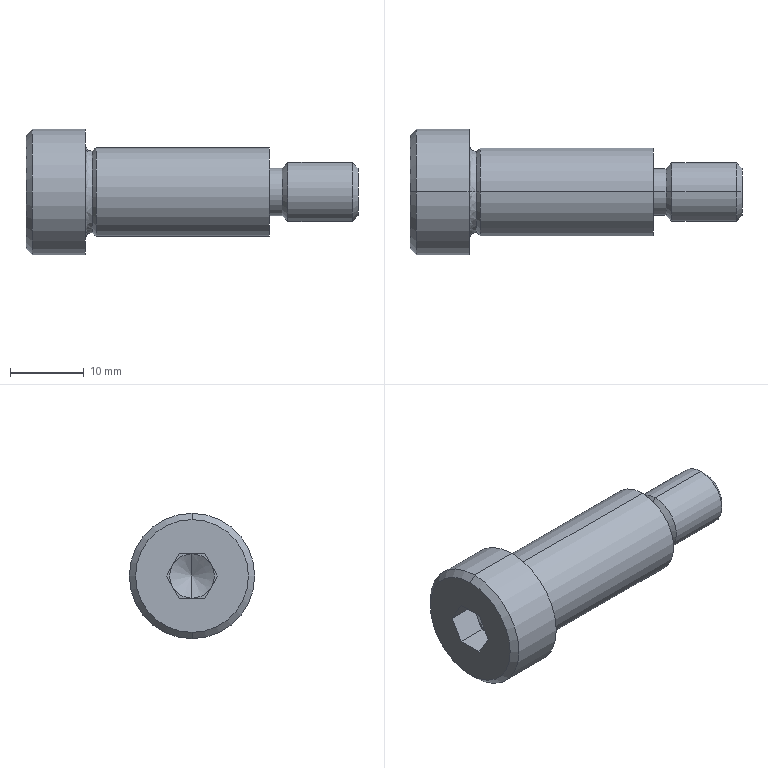Part | STEP file | 0228_002_MSB12-25 | 1 solid | 36 faces | box 45 x 17 x 17 mm | volume 5025 mm3 | plane 16 | cone 10 | cylinder 8 | spline 2 | commonest cylinder face diameters 6.4 x2 8 x2 12 x2 17 x2